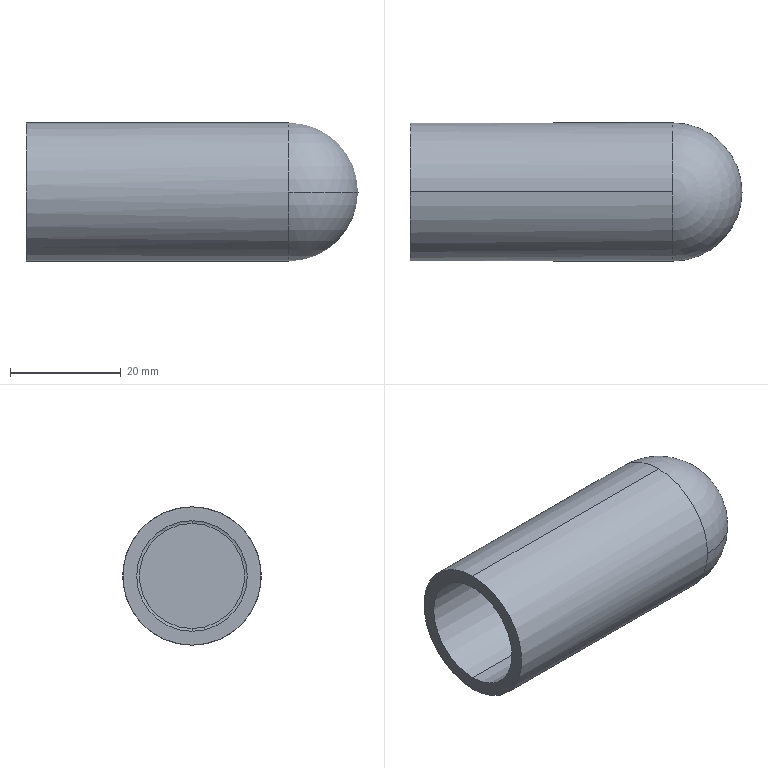Part | SolidWorks | features ICE 2, Fillet 1, Revolution 1 | 1 solid | 14 faces | box 60 x 25 x 25 mm | volume 11560 mm3 | cylinder 6 | torus 4 | sphere 2 | plane 2 | commonest cylinder face diameters 20 x2 21 x2 25 x2
STEP:
#1=CARTESIAN_POINT('',(50.,0.,-9.5));
#2=VERTEX_POINT('',#1);
#3=CARTESIAN_POINT('',(50.,0.,9.5));
#4=VERTEX_POINT('',#3);
#5=CARTESIAN_POINT('',(50.,0.,0.));
#6=DIRECTION('',(-1.,0.,0.));
#7=DIRECTION('',(0.,0.,1.));
#8=AXIS2_PLACEMENT_3D('',#5,#6,#7);
#9=CIRCLE('',#8,9.5);
#10=EDGE_CURVE('',#2,#4,#9,.T.);
#11=ORIENTED_EDGE('',*,*,#10,.F.);
#12=CARTESIAN_POINT('',(49.,0.,-10.5));
#13=VERTEX_POINT('',#12);
#14=CARTESIAN_POINT('',(49.,0.,-9.5));
#15=DIRECTION('',(0.,1.,0.));
#16=DIRECTION('',(0.,0.,1.));
#17=AXIS2_PLACEMENT_3D('',#14,#15,#16);
#18=CIRCLE('',#17,1.);
#19=EDGE_CURVE('',#2,#13,#18,.T.);
#20=ORIENTED_EDGE('',*,*,#19,.T.);
#21=CARTESIAN_POINT('',(49.,0.,10.5));
#22=VERTEX_POINT('',#21);
#23=CARTESIAN_POINT('',(49.,0.,0.));
#24=DIRECTION('',(1.,0.,0.));
#25=DIRECTION('',(0.,0.,1.));
#26=AXIS2_PLACEMENT_3D('',#23,#24,#25);
#27=CIRCLE('',#26,10.5);
#28=EDGE_CURVE('',#22,#13,#27,.T.);
#29=ORIENTED_EDGE('',*,*,#28,.F.);
#30=CARTESIAN_POINT('',(49.,0.,9.5));
#31=DIRECTION('',(0.,-1.,0.));
#32=DIRECTION('',(0.,0.,-1.));
#33=AXIS2_PLACEMENT_3D('',#30,#31,#32);
#34=CIRCLE('',#33,1.);
#35=EDGE_CURVE('',#4,#22,#34,.T.);
#36=ORIENTED_EDGE('',*,*,#35,.F.);
#37=EDGE_LOOP('',(#11,#20,#29,#36));
#38=FACE_OUTER_BOUND('',#37,.T.);
#39=CARTESIAN_POINT('',(49.,0.,0.));
#40=DIRECTION('',(-1.,0.,0.));
#41=DIRECTION('',(0.,0.,1.));
#42=AXIS2_PLACEMENT_3D('',#39,#40,#41);
#43=TOROIDAL_SURFACE('',#42,9.5,1.);
#44=ADVANCED_FACE('',(#38),#43,.F.);
#45=CARTESIAN_POINT('',(45.866,0.,-10.5));
#46=VERTEX_POINT('',#45);
#47=CARTESIAN_POINT('',(45.866,0.,10.5));
#48=VERTEX_POINT('',#47);
#49=CARTESIAN_POINT('',(45.866,0.,0.));
#50=DIRECTION('',(-1.,0.,0.));
#51=DIRECTION('',(0.,0.,1.));
#52=AXIS2_PLACEMENT_3D('',#49,#50,#51);
#53=CIRCLE('',#52,10.5);
#54=EDGE_CURVE('',#46,#48,#53,.T.);
#55=ORIENTED_EDGE('',*,*,#54,.F.);
#56=CARTESIAN_POINT('',(45.,0.,-10.));
#57=VERTEX_POINT('',#56);
#58=CARTESIAN_POINT('',(45.866,0.,-9.5));
#59=DIRECTION('',(0.,1.,0.));
#60=DIRECTION('',(0.,0.,1.));
#61=AXIS2_PLACEMENT_3D('',#58,#59,#60);
#62=CIRCLE('',#61,1.);
#63=EDGE_CURVE('',#46,#57,#62,.T.);
#64=ORIENTED_EDGE('',*,*,#63,.T.);
#65=CARTESIAN_POINT('',(45.,0.,10.));
#66=VERTEX_POINT('',#65);
#67=CARTESIAN_POINT('',(45.,0.,0.));
#68=DIRECTION('',(-1.,0.,0.));
#69=DIRECTION('',(0.,0.,1.));
#70=AXIS2_PLACEMENT_3D('',#67,#68,#69);
#71=CIRCLE('',#70,10.);
#72=EDGE_CURVE('',#57,#66,#71,.T.);
#73=ORIENTED_EDGE('',*,*,#72,.T.);
#74=CARTESIAN_POINT('',(45.866,0.,9.5));
#75=DIRECTION('',(0.,-1.,0.));
#76=DIRECTION('',(0.,0.,-1.));
#77=AXIS2_PLACEMENT_3D('',#74,#75,#76);
#78=CIRCLE('',#77,1.);
#79=EDGE_CURVE('',#48,#66,#78,.T.);
#80=ORIENTED_EDGE('',*,*,#79,.F.);
#81=EDGE_LOOP('',(#55,#64,#73,#80));
#82=FACE_OUTER_BOUND('',#81,.T.);
#83=CARTESIAN_POINT('',(45.866,0.,0.));
#84=DIRECTION('',(-1.,0.,0.));
#85=DIRECTION('',(0.,0.,1.));
#86=AXIS2_PLACEMENT_3D('',#83,#84,#85);
#87=TOROIDAL_SURFACE('',#86,9.5,1.);
#88=ADVANCED_FACE('',(#82),#87,.F.);
#89=ORIENTED_EDGE('',*,*,#54,.T.);
#90=CARTESIAN_POINT('',(15.302,0.,10.5));
#91=DIRECTION('',(1.,0.,0.));
#92=VECTOR('',#91,1000.);
#93=LINE('',#90,#92);
#94=EDGE_CURVE('',#48,#22,#93,.T.);
#95=ORIENTED_EDGE('',*,*,#94,.T.);
#96=ORIENTED_EDGE('',*,*,#28,.T.);
#97=CARTESIAN_POINT('',(15.302,0.,-10.5));
#98=DIRECTION('',(1.,0.,0.));
#99=VECTOR('',#98,1000.);
#100=LINE('',#97,#99);
#101=EDGE_CURVE('',#46,#13,#100,.T.);
#102=ORIENTED_EDGE('',*,*,#101,.F.);
#103=EDGE_LOOP('',(#89,#95,#96,#102));
#104=FACE_OUTER_BOUND('',#103,.T.);
#105=CARTESIAN_POINT('',(15.302,0.,0.));
#106=DIRECTION('',(1.,0.,0.));
#107=DIRECTION('',(0.,0.,-1.));
#108=AXIS2_PLACEMENT_3D('',#105,#106,#107);
#109=CYLINDRICAL_SURFACE('',#108,10.5);
#110=ADVANCED_FACE('',(#104),#109,.F.);
#111=ORIENTED_EDGE('',*,*,#72,.F.);
#112=CARTESIAN_POINT('',(0.,0.,-10.));
#113=VERTEX_POINT('',#112);
#114=CARTESIAN_POINT('',(45.,0.,-10.));
#115=DIRECTION('',(-1.,0.,0.));
#116=VECTOR('',#115,1000.);
#117=LINE('',#114,#116);
#118=EDGE_CURVE('',#57,#113,#117,.T.);
#119=ORIENTED_EDGE('',*,*,#118,.T.);
#120=CARTESIAN_POINT('',(0.,0.,10.));
#121=VERTEX_POINT('',#120);
#122=CARTESIAN_POINT('',(0.,0.,0.));
#123=DIRECTION('',(-1.,0.,0.));
#124=DIRECTION('',(0.,0.,1.));
#125=AXIS2_PLACEMENT_3D('',#122,#123,#124);
#126=CIRCLE('',#125,10.);
#127=EDGE_CURVE('',#113,#121,#126,.T.);
#128=ORIENTED_EDGE('',*,*,#127,.T.);
#129=CARTESIAN_POINT('',(45.,0.,10.));
#130=DIRECTION('',(-1.,0.,0.));
#131=VECTOR('',#130,1000.);
#132=LINE('',#129,#131);
#133=EDGE_CURVE('',#66,#121,#132,.T.);
#134=ORIENTED_EDGE('',*,*,#133,.F.);
#135=EDGE_LOOP('',(#111,#119,#128,#134));
#136=FACE_OUTER_BOUND('',#135,.T.);
#137=CARTESIAN_POINT('',(45.,0.,0.));
#138=DIRECTION('',(-1.,0.,0.));
#139=DIRECTION('',(0.,0.,1.));
#140=AXIS2_PLACEMENT_3D('',#137,#138,#139);
#141=CYLINDRICAL_SURFACE('',#140,10.);
#142=ADVANCED_FACE('',(#136),#141,.F.);
#143=CARTESIAN_POINT('',(60.,0.,0.));
#144=VERTEX_POINT('',#143);
#145=CARTESIAN_POINT('',(47.5,12.5,0.));
#146=VERTEX_POINT('',#145);
#147=CARTESIAN_POINT('',(47.5,0.,0.));
#148=DIRECTION('',(0.,0.,1.));
#149=DIRECTION('',(1.,0.,0.));
#150=AXIS2_PLACEMENT_3D('',#147,#148,#149);
#151=CIRCLE('',#150,12.5);
#152=EDGE_CURVE('',#144,#146,#151,.T.);
#153=ORIENTED_EDGE('',*,*,#152,.F.);
#154=CARTESIAN_POINT('',(47.5,-12.5,0.));
#155=VERTEX_POINT('',#154);
#156=CARTESIAN_POINT('',(47.5,0.,0.));
#157=DIRECTION('',(0.,0.,-1.));
#158=DIRECTION('',(0.,1.,0.));
#159=AXIS2_PLACEMENT_3D('',#156,#157,#158);
#160=CIRCLE('',#159,12.5);
#161=EDGE_CURVE('',#144,#155,#160,.T.);
#162=ORIENTED_EDGE('',*,*,#161,.T.);
#163=CARTESIAN_POINT('',(47.5,0.,-12.5));
#164=VERTEX_POINT('',#163);
#165=CARTESIAN_POINT('',(47.5,0.,0.));
#166=DIRECTION('',(-1.,0.,0.));
#167=DIRECTION('',(0.,0.,1.));
#168=AXIS2_PLACEMENT_3D('',#165,#166,#167);
#169=CIRCLE('',#168,12.5);
#170=EDGE_CURVE('',#164,#155,#169,.T.);
#171=ORIENTED_EDGE('',*,*,#170,.F.);
#172=CARTESIAN_POINT('',(47.5,0.,0.));
#173=DIRECTION('',(-1.,0.,0.));
#174=DIRECTION('',(0.,0.,1.));
#175=AXIS2_PLACEMENT_3D('',#172,#173,#174);
#176=CIRCLE('',#175,12.5);
#177=EDGE_CURVE('',#146,#164,#176,.T.);
#178=ORIENTED_EDGE('',*,*,#177,.F.);
#179=EDGE_LOOP('',(#153,#162,#171,#178));
#180=FACE_OUTER_BOUND('',#179,.T.);
#181=CARTESIAN_POINT('',(47.5,0.,0.));
#182=DIRECTION('',(0.,0.,-1.));
#183=DIRECTION('',(0.,1.,0.));
#184=AXIS2_PLACEMENT_3D('',#181,#182,#183);
#185=SPHERICAL_SURFACE('',#184,12.5);
#186=ADVANCED_FACE('',(#180),#185,.T.);
#187=CARTESIAN_POINT('',(47.5,0.,12.5));
#188=VERTEX_POINT('',#187);
#189=CARTESIAN_POINT('',(47.5,0.,0.));
#190=DIRECTION('',(-1.,0.,0.));
#191=DIRECTION('',(0.,0.,1.));
#192=AXIS2_PLACEMENT_3D('',#189,#190,#191);
#193=CIRCLE('',#192,12.5);
#194=EDGE_CURVE('',#188,#146,#193,.T.);
#195=ORIENTED_EDGE('',*,*,#194,.T.);
#196=ORIENTED_EDGE('',*,*,#177,.T.);
#197=CARTESIAN_POINT('',(0.,0.,-12.5));
#198=VERTEX_POINT('',#197);
#199=CARTESIAN_POINT('',(0.,0.,-12.5));
#200=DIRECTION('',(-1.,0.,0.));
#201=VECTOR('',#200,1000.);
#202=LINE('',#199,#201);
#203=EDGE_CURVE('',#164,#198,#202,.T.);
#204=ORIENTED_EDGE('',*,*,#203,.T.);
#205=CARTESIAN_POINT('',(0.,0.,12.5));
#206=VERTEX_POINT('',#205);
#207=CARTESIAN_POINT('',(0.,0.,0.));
#208=DIRECTION('',(-1.,0.,0.));
#209=DIRECTION('',(0.,0.,1.));
#210=AXIS2_PLACEMENT_3D('',#207,#208,#209);
#211=CIRCLE('',#210,12.5);
#212=EDGE_CURVE('',#206,#198,#211,.T.);
#213=ORIENTED_EDGE('',*,*,#212,.F.);
#214=CARTESIAN_POINT('',(0.,0.,12.5));
#215=DIRECTION('',(-1.,0.,0.));
#216=VECTOR('',#215,1000.);
#217=LINE('',#214,#216);
#218=EDGE_CURVE('',#188,#206,#217,.T.);
#219=ORIENTED_EDGE('',*,*,#218,.F.);
#220=EDGE_LOOP('',(#195,#196,#204,#213,#219));
#221=FACE_OUTER_BOUND('',#220,.T.);
#222=CARTESIAN_POINT('',(0.,0.,0.));
#223=DIRECTION('',(-1.,0.,0.));
#224=DIRECTION('',(0.,0.,1.));
#225=AXIS2_PLACEMENT_3D('',#222,#223,#224);
#226=CYLINDRICAL_SURFACE('',#225,12.5);
#227=ADVANCED_FACE('',(#221),#226,.T.);
#228=CARTESIAN_POINT('',(0.,0.,0.));
#229=DIRECTION('',(-1.,0.,0.));
#230=DIRECTION('',(0.,0.,1.));
#231=AXIS2_PLACEMENT_3D('',#228,#229,#230);
#232=CIRCLE('',#231,10.);
#233=EDGE_CURVE('',#121,#113,#232,.T.);
#234=ORIENTED_EDGE('',*,*,#233,.F.);
#235=ORIENTED_EDGE('',*,*,#127,.F.);
#236=EDGE_LOOP('',(#234,#235));
#237=FACE_BOUND('',#236,.T.);
#238=ORIENTED_EDGE('',*,*,#212,.T.);
#239=CARTESIAN_POINT('',(0.,0.,0.));
#240=DIRECTION('',(-1.,0.,0.));
#241=DIRECTION('',(0.,0.,1.));
#242=AXIS2_PLACEMENT_3D('',#239,#240,#241);
#243=CIRCLE('',#242,12.5);
#244=EDGE_CURVE('',#198,#206,#243,.T.);
#245=ORIENTED_EDGE('',*,*,#244,.T.);
#246=EDGE_LOOP('',(#238,#245));
#247=FACE_OUTER_BOUND('',#246,.T.);
#248=CARTESIAN_POINT('',(0.,0.,0.));
#249=DIRECTION('',(1.,0.,0.));
#250=DIRECTION('',(0.,0.,-1.));
#251=AXIS2_PLACEMENT_3D('',#248,#249,#250);
#252=PLANE('',#251);
#253=ADVANCED_FACE('',(#237,#247),#252,.F.);
#254=ORIENTED_EDGE('',*,*,#203,.F.);
#255=ORIENTED_EDGE('',*,*,#170,.T.);
#256=CARTESIAN_POINT('',(47.5,0.,0.));
#257=DIRECTION('',(-1.,0.,0.));
#258=DIRECTION('',(0.,0.,1.));
#259=AXIS2_PLACEMENT_3D('',#256,#257,#258);
#260=CIRCLE('',#259,12.5);
#261=EDGE_CURVE('',#155,#188,#260,.T.);
#262=ORIENTED_EDGE('',*,*,#261,.T.);
#263=ORIENTED_EDGE('',*,*,#218,.T.);
#264=ORIENTED_EDGE('',*,*,#244,.F.);
#265=EDGE_LOOP('',(#254,#255,#262,#263,#264));
#266=FACE_OUTER_BOUND('',#265,.T.);
#267=CARTESIAN_POINT('',(0.,0.,0.));
#268=DIRECTION('',(-1.,0.,0.));
#269=DIRECTION('',(0.,0.,1.));
#270=AXIS2_PLACEMENT_3D('',#267,#268,#269);
#271=CYLINDRICAL_SURFACE('',#270,12.5);
#272=ADVANCED_FACE('',(#266),#271,.T.);
#273=ORIENTED_EDGE('',*,*,#161,.F.);
#274=ORIENTED_EDGE('',*,*,#152,.T.);
#275=ORIENTED_EDGE('',*,*,#194,.F.);
#276=ORIENTED_EDGE('',*,*,#261,.F.);
#277=EDGE_LOOP('',(#273,#274,#275,#276));
#278=FACE_OUTER_BOUND('',#277,.T.);
#279=CARTESIAN_POINT('',(47.5,0.,0.));
#280=DIRECTION('',(0.,0.,-1.));
#281=DIRECTION('',(0.,1.,0.));
#282=AXIS2_PLACEMENT_3D('',#279,#280,#281);
#283=SPHERICAL_SURFACE('',#282,12.5);
#284=ADVANCED_FACE('',(#278),#283,.T.);
#285=ORIENTED_EDGE('',*,*,#118,.F.);
#286=CARTESIAN_POINT('',(45.,0.,0.));
#287=DIRECTION('',(-1.,0.,0.));
#288=DIRECTION('',(0.,0.,1.));
#289=AXIS2_PLACEMENT_3D('',#286,#287,#288);
#290=CIRCLE('',#289,10.);
#291=EDGE_CURVE('',#66,#57,#290,.T.);
#292=ORIENTED_EDGE('',*,*,#291,.F.);
#293=ORIENTED_EDGE('',*,*,#133,.T.);
#294=ORIENTED_EDGE('',*,*,#233,.T.);
#295=EDGE_LOOP('',(#285,#292,#293,#294));
#296=FACE_OUTER_BOUND('',#295,.T.);
#297=CARTESIAN_POINT('',(45.,0.,0.));
#298=DIRECTION('',(-1.,0.,0.));
#299=DIRECTION('',(0.,0.,1.));
#300=AXIS2_PLACEMENT_3D('',#297,#298,#299);
#301=CYLINDRICAL_SURFACE('',#300,10.);
#302=ADVANCED_FACE('',(#296),#301,.F.);
#303=ORIENTED_EDGE('',*,*,#94,.F.);
#304=CARTESIAN_POINT('',(45.866,0.,0.));
#305=DIRECTION('',(-1.,0.,0.));
#306=DIRECTION('',(0.,0.,1.));
#307=AXIS2_PLACEMENT_3D('',#304,#305,#306);
#308=CIRCLE('',#307,10.5);
#309=EDGE_CURVE('',#48,#46,#308,.T.);
#310=ORIENTED_EDGE('',*,*,#309,.T.);
#311=ORIENTED_EDGE('',*,*,#101,.T.);
#312=CARTESIAN_POINT('',(49.,0.,0.));
#313=DIRECTION('',(1.,0.,0.));
#314=DIRECTION('',(0.,0.,1.));
#315=AXIS2_PLACEMENT_3D('',#312,#313,#314);
#316=CIRCLE('',#315,10.5);
#317=EDGE_CURVE('',#13,#22,#316,.T.);
#318=ORIENTED_EDGE('',*,*,#317,.T.);
#319=EDGE_LOOP('',(#303,#310,#311,#318));
#320=FACE_OUTER_BOUND('',#319,.T.);
#321=CARTESIAN_POINT('',(15.302,0.,0.));
#322=DIRECTION('',(1.,0.,0.));
#323=DIRECTION('',(0.,0.,-1.));
#324=AXIS2_PLACEMENT_3D('',#321,#322,#323);
#325=CYLINDRICAL_SURFACE('',#324,10.5);
#326=ADVANCED_FACE('',(#320),#325,.F.);
#327=CARTESIAN_POINT('',(50.,0.,0.));
#328=DIRECTION('',(-1.,0.,0.));
#329=DIRECTION('',(0.,0.,1.));
#330=AXIS2_PLACEMENT_3D('',#327,#328,#329);
#331=CIRCLE('',#330,9.5);
#332=EDGE_CURVE('',#4,#2,#331,.T.);
#333=ORIENTED_EDGE('',*,*,#332,.T.);
#334=ORIENTED_EDGE('',*,*,#10,.T.);
#335=EDGE_LOOP('',(#333,#334));
#336=FACE_OUTER_BOUND('',#335,.T.);
#337=CARTESIAN_POINT('',(50.,0.,0.));
#338=DIRECTION('',(-1.,0.,0.));
#339=DIRECTION('',(0.,0.,1.));
#340=AXIS2_PLACEMENT_3D('',#337,#338,#339);
#341=PLANE('',#340);
#342=ADVANCED_FACE('',(#336),#341,.T.);
#343=ORIENTED_EDGE('',*,*,#63,.F.);
#344=ORIENTED_EDGE('',*,*,#309,.F.);
#345=ORIENTED_EDGE('',*,*,#79,.T.);
#346=ORIENTED_EDGE('',*,*,#291,.T.);
#347=EDGE_LOOP('',(#343,#344,#345,#346));
#348=FACE_OUTER_BOUND('',#347,.T.);
#349=CARTESIAN_POINT('',(45.866,0.,0.));
#350=DIRECTION('',(-1.,0.,0.));
#351=DIRECTION('',(0.,0.,1.));
#352=AXIS2_PLACEMENT_3D('',#349,#350,#351);
#353=TOROIDAL_SURFACE('',#352,9.5,1.);
#354=ADVANCED_FACE('',(#348),#353,.F.);
#355=ORIENTED_EDGE('',*,*,#19,.F.);
#356=ORIENTED_EDGE('',*,*,#332,.F.);
#357=ORIENTED_EDGE('',*,*,#35,.T.);
#358=ORIENTED_EDGE('',*,*,#317,.F.);
#359=EDGE_LOOP('',(#355,#356,#357,#358));
#360=FACE_OUTER_BOUND('',#359,.T.);
#361=CARTESIAN_POINT('',(49.,0.,0.));
#362=DIRECTION('',(-1.,0.,0.));
#363=DIRECTION('',(0.,0.,1.));
#364=AXIS2_PLACEMENT_3D('',#361,#362,#363);
#365=TOROIDAL_SURFACE('',#364,9.5,1.);
#366=ADVANCED_FACE('',(#360),#365,.F.);
#367=CLOSED_SHELL('',(#44,#88,#110,#142,#186,#227,#253,#272,#284,#302,#326,#342,#354,#366));
#368=MANIFOLD_SOLID_BREP('',#367);
#369=CARTESIAN_POINT('',(0.,0.,0.));
#370=DIRECTION('',(0.,0.,1.));
#371=DIRECTION('',(1.,0.,0.));
#372=AXIS2_PLACEMENT_3D('',#369,#370,#371);
#373=(LENGTH_UNIT()NAMED_UNIT(*)SI_UNIT(.MILLI.,.METRE.));
#374=UNCERTAINTY_MEASURE_WITH_UNIT(LENGTH_MEASURE(0.00001),#373,'','');
#375=(NAMED_UNIT(*)PLANE_ANGLE_UNIT()SI_UNIT($,.RADIAN.));
#376=(NAMED_UNIT(*)SI_UNIT($,.STERADIAN.)SOLID_ANGLE_UNIT());
#377=(GEOMETRIC_REPRESENTATION_CONTEXT(3)GLOBAL_UNCERTAINTY_ASSIGNED_CONTEXT((#374))GLOBAL_UNIT_ASSIGNED_CONTEXT((#373,#375,#376))REPRESENTATION_CONTEXT('',''));
#378=ADVANCED_BREP_SHAPE_REPRESENTATION('',(#368,#372),#377);